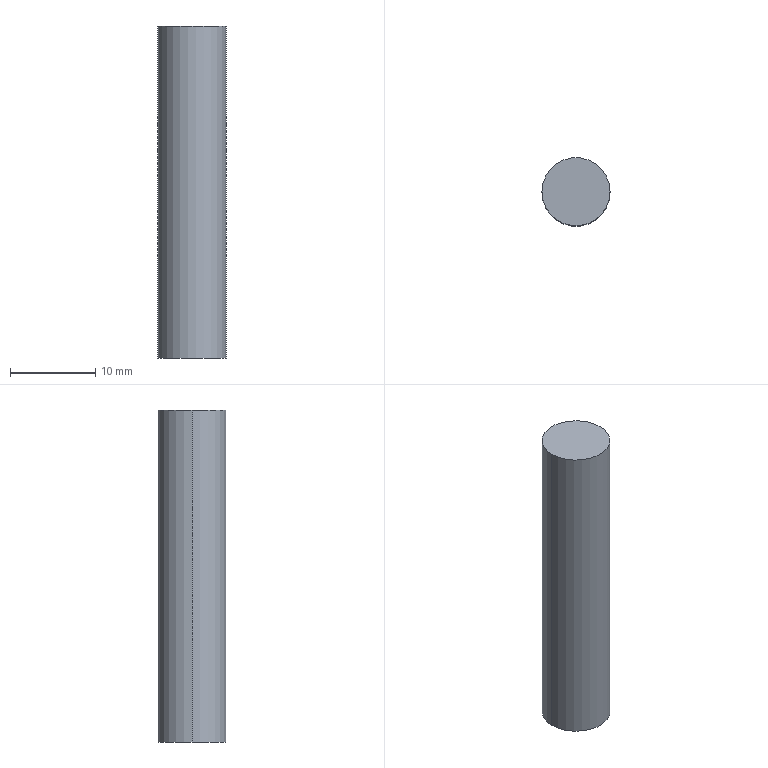Part | SolidWorks | features Extrusion 1 | 1 solid | 4 faces | box 8 x 8 x 39 mm | volume 1960 mm3 | cylinder 2 | plane 2 | commonest cylinder face diameters 8 x2
STEP:
#1=CARTESIAN_POINT('',(4.,0.,39.));
#2=VERTEX_POINT('',#1);
#3=CARTESIAN_POINT('',(-4.,0.,39.));
#4=VERTEX_POINT('',#3);
#5=CARTESIAN_POINT('',(0.,0.,39.));
#6=DIRECTION('',(0.,0.,1.));
#7=DIRECTION('',(1.,0.,0.));
#8=AXIS2_PLACEMENT_3D('',#5,#6,#7);
#9=CIRCLE('',#8,4.);
#10=EDGE_CURVE('',#2,#4,#9,.T.);
#11=ORIENTED_EDGE('',*,*,#10,.F.);
#12=CARTESIAN_POINT('',(4.,0.,0.));
#13=VERTEX_POINT('',#12);
#14=CARTESIAN_POINT('',(4.,0.,39.));
#15=DIRECTION('',(0.,0.,-1.));
#16=VECTOR('',#15,1000.);
#17=LINE('',#14,#16);
#18=EDGE_CURVE('',#2,#13,#17,.T.);
#19=ORIENTED_EDGE('',*,*,#18,.T.);
#20=CARTESIAN_POINT('',(-4.,0.,0.));
#21=VERTEX_POINT('',#20);
#22=CARTESIAN_POINT('',(0.,0.,0.));
#23=DIRECTION('',(0.,0.,1.));
#24=DIRECTION('',(1.,0.,0.));
#25=AXIS2_PLACEMENT_3D('',#22,#23,#24);
#26=CIRCLE('',#25,4.);
#27=EDGE_CURVE('',#13,#21,#26,.T.);
#28=ORIENTED_EDGE('',*,*,#27,.T.);
#29=CARTESIAN_POINT('',(-4.,0.,39.));
#30=DIRECTION('',(0.,0.,-1.));
#31=VECTOR('',#30,1000.);
#32=LINE('',#29,#31);
#33=EDGE_CURVE('',#4,#21,#32,.T.);
#34=ORIENTED_EDGE('',*,*,#33,.F.);
#35=EDGE_LOOP('',(#11,#19,#28,#34));
#36=FACE_OUTER_BOUND('',#35,.T.);
#37=CARTESIAN_POINT('',(0.,0.,39.));
#38=DIRECTION('',(0.,0.,-1.));
#39=DIRECTION('',(-1.,0.,0.));
#40=AXIS2_PLACEMENT_3D('',#37,#38,#39);
#41=CYLINDRICAL_SURFACE('',#40,4.);
#42=ADVANCED_FACE('',(#36),#41,.T.);
#43=ORIENTED_EDGE('',*,*,#18,.F.);
#44=CARTESIAN_POINT('',(0.,0.,39.));
#45=DIRECTION('',(0.,0.,1.));
#46=DIRECTION('',(1.,0.,0.));
#47=AXIS2_PLACEMENT_3D('',#44,#45,#46);
#48=CIRCLE('',#47,4.);
#49=EDGE_CURVE('',#4,#2,#48,.T.);
#50=ORIENTED_EDGE('',*,*,#49,.F.);
#51=ORIENTED_EDGE('',*,*,#33,.T.);
#52=CARTESIAN_POINT('',(0.,0.,0.));
#53=DIRECTION('',(0.,0.,1.));
#54=DIRECTION('',(1.,0.,0.));
#55=AXIS2_PLACEMENT_3D('',#52,#53,#54);
#56=CIRCLE('',#55,4.);
#57=EDGE_CURVE('',#21,#13,#56,.T.);
#58=ORIENTED_EDGE('',*,*,#57,.T.);
#59=EDGE_LOOP('',(#43,#50,#51,#58));
#60=FACE_OUTER_BOUND('',#59,.T.);
#61=CARTESIAN_POINT('',(0.,0.,39.));
#62=DIRECTION('',(0.,0.,-1.));
#63=DIRECTION('',(-1.,0.,0.));
#64=AXIS2_PLACEMENT_3D('',#61,#62,#63);
#65=CYLINDRICAL_SURFACE('',#64,4.);
#66=ADVANCED_FACE('',(#60),#65,.T.);
#67=ORIENTED_EDGE('',*,*,#49,.T.);
#68=ORIENTED_EDGE('',*,*,#10,.T.);
#69=EDGE_LOOP('',(#67,#68));
#70=FACE_OUTER_BOUND('',#69,.T.);
#71=CARTESIAN_POINT('',(0.,0.,39.));
#72=DIRECTION('',(0.,0.,1.));
#73=DIRECTION('',(1.,0.,0.));
#74=AXIS2_PLACEMENT_3D('',#71,#72,#73);
#75=PLANE('',#74);
#76=ADVANCED_FACE('',(#70),#75,.T.);
#77=ORIENTED_EDGE('',*,*,#57,.F.);
#78=ORIENTED_EDGE('',*,*,#27,.F.);
#79=EDGE_LOOP('',(#77,#78));
#80=FACE_OUTER_BOUND('',#79,.T.);
#81=CARTESIAN_POINT('',(0.,0.,0.));
#82=DIRECTION('',(0.,0.,1.));
#83=DIRECTION('',(1.,0.,0.));
#84=AXIS2_PLACEMENT_3D('',#81,#82,#83);
#85=PLANE('',#84);
#86=ADVANCED_FACE('',(#80),#85,.F.);
#87=CLOSED_SHELL('',(#42,#66,#76,#86));
#88=MANIFOLD_SOLID_BREP('',#87);
#89=CARTESIAN_POINT('',(0.,0.,0.));
#90=DIRECTION('',(0.,0.,1.));
#91=DIRECTION('',(1.,0.,0.));
#92=AXIS2_PLACEMENT_3D('',#89,#90,#91);
#93=(LENGTH_UNIT()NAMED_UNIT(*)SI_UNIT(.MILLI.,.METRE.));
#94=UNCERTAINTY_MEASURE_WITH_UNIT(LENGTH_MEASURE(0.00001),#93,'','');
#95=(NAMED_UNIT(*)PLANE_ANGLE_UNIT()SI_UNIT($,.RADIAN.));
#96=(NAMED_UNIT(*)SI_UNIT($,.STERADIAN.)SOLID_ANGLE_UNIT());
#97=(GEOMETRIC_REPRESENTATION_CONTEXT(3)GLOBAL_UNCERTAINTY_ASSIGNED_CONTEXT((#94))GLOBAL_UNIT_ASSIGNED_CONTEXT((#93,#95,#96))REPRESENTATION_CONTEXT('',''));
#98=ADVANCED_BREP_SHAPE_REPRESENTATION('',(#88,#92),#97);